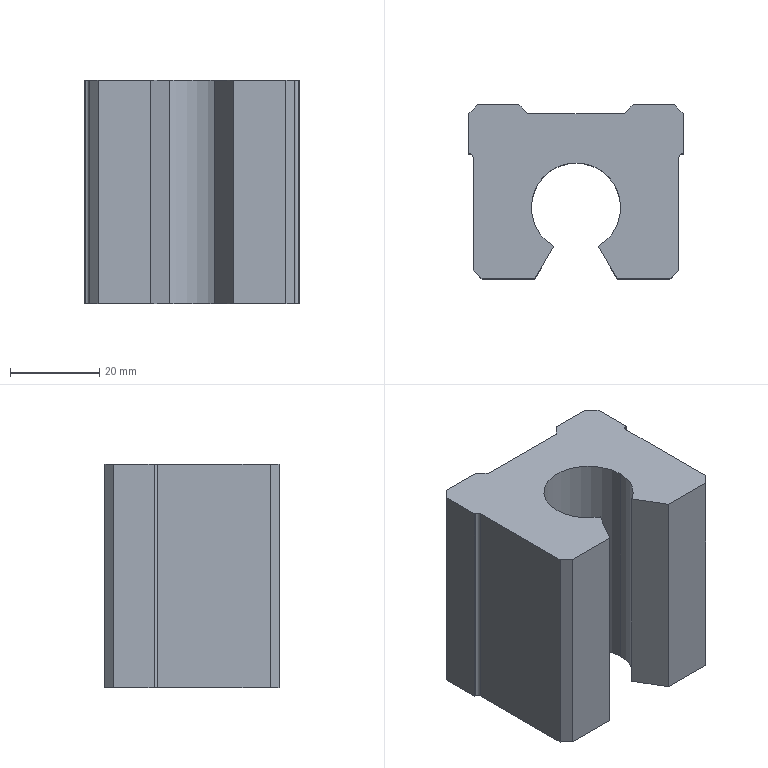Part | SolidWorks | features Chamfer 1, Extrusion 1, ICE 1 | 1 solid | 42 faces | box 48 x 39 x 50 mm | volume 66905 mm3 | plane 21 | cylinder 13 | cone 8 | commonest cylinder face diameters 4.891 x8 20 x3 1.536 x2
STEP:
#1=CARTESIAN_POINT('',(17.5,38.,-42.5));
#2=VERTEX_POINT('',#1);
#3=CARTESIAN_POINT('',(17.5,40.445,-40.054));
#4=VERTEX_POINT('',#3);
#5=CARTESIAN_POINT('',(17.5,40.445,-40.054));
#6=DIRECTION('',(0.,0.7071,0.7071));
#7=VECTOR('',#6,1000.);
#8=LINE('',#5,#7);
#9=EDGE_CURVE('',#2,#4,#8,.T.);
#10=ORIENTED_EDGE('',*,*,#9,.F.);
#11=CARTESIAN_POINT('',(17.5,40.445,-44.945));
#12=VERTEX_POINT('',#11);
#13=CARTESIAN_POINT('',(17.5,40.445,-44.945));
#14=DIRECTION('',(0.,0.7071,-0.7071));
#15=VECTOR('',#14,1000.);
#16=LINE('',#13,#15);
#17=EDGE_CURVE('',#2,#12,#16,.T.);
#18=ORIENTED_EDGE('',*,*,#17,.T.);
#19=CARTESIAN_POINT('',(17.5,40.445,-42.5));
#20=DIRECTION('',(0.,-1.,0.));
#21=DIRECTION('',(0.,0.,1.));
#22=AXIS2_PLACEMENT_3D('',#19,#20,#21);
#23=CIRCLE('',#22,2.445);
#24=EDGE_CURVE('',#4,#12,#23,.T.);
#25=ORIENTED_EDGE('',*,*,#24,.F.);
#26=EDGE_LOOP('',(#10,#18,#25));
#27=FACE_OUTER_BOUND('',#26,.T.);
#28=CARTESIAN_POINT('',(17.5,40.445,-42.5));
#29=DIRECTION('',(0.,1.,0.));
#30=DIRECTION('',(0.,0.,1.));
#31=AXIS2_PLACEMENT_3D('',#28,#29,#30);
#32=CONICAL_SURFACE('',#31,2.446,0.7854);
#33=ADVANCED_FACE('',(#27),#32,.F.);
#34=CARTESIAN_POINT('',(-17.5,38.,-42.5));
#35=VERTEX_POINT('',#34);
#36=CARTESIAN_POINT('',(-17.5,40.445,-40.055));
#37=VERTEX_POINT('',#36);
#38=CARTESIAN_POINT('',(-17.5,40.445,-40.055));
#39=DIRECTION('',(0.,0.7071,0.7071));
#40=VECTOR('',#39,1000.);
#41=LINE('',#38,#40);
#42=EDGE_CURVE('',#35,#37,#41,.T.);
#43=ORIENTED_EDGE('',*,*,#42,.F.);
#44=CARTESIAN_POINT('',(-17.5,40.445,-44.946));
#45=VERTEX_POINT('',#44);
#46=CARTESIAN_POINT('',(-17.5,40.445,-44.946));
#47=DIRECTION('',(0.,0.7071,-0.7071));
#48=VECTOR('',#47,1000.);
#49=LINE('',#46,#48);
#50=EDGE_CURVE('',#35,#45,#49,.T.);
#51=ORIENTED_EDGE('',*,*,#50,.T.);
#52=CARTESIAN_POINT('',(-17.5,40.445,-42.5));
#53=DIRECTION('',(0.,-1.,0.));
#54=DIRECTION('',(0.,0.,1.));
#55=AXIS2_PLACEMENT_3D('',#52,#53,#54);
#56=CIRCLE('',#55,2.446);
#57=EDGE_CURVE('',#37,#45,#56,.T.);
#58=ORIENTED_EDGE('',*,*,#57,.F.);
#59=EDGE_LOOP('',(#43,#51,#58));
#60=FACE_OUTER_BOUND('',#59,.T.);
#61=CARTESIAN_POINT('',(-17.5,40.445,-42.5));
#62=DIRECTION('',(0.,1.,0.));
#63=DIRECTION('',(0.,0.,1.));
#64=AXIS2_PLACEMENT_3D('',#61,#62,#63);
#65=CONICAL_SURFACE('',#64,2.446,0.7854);
#66=ADVANCED_FACE('',(#60),#65,.F.);
#67=CARTESIAN_POINT('',(-17.5,38.,-7.5));
#68=VERTEX_POINT('',#67);
#69=CARTESIAN_POINT('',(-17.5,40.446,-5.054));
#70=VERTEX_POINT('',#69);
#71=CARTESIAN_POINT('',(-17.5,40.446,-5.054));
#72=DIRECTION('',(0.,0.7071,0.7071));
#73=VECTOR('',#72,1000.);
#74=LINE('',#71,#73);
#75=EDGE_CURVE('',#68,#70,#74,.T.);
#76=ORIENTED_EDGE('',*,*,#75,.F.);
#77=CARTESIAN_POINT('',(-17.5,40.446,-9.945));
#78=VERTEX_POINT('',#77);
#79=CARTESIAN_POINT('',(-17.5,40.446,-9.945));
#80=DIRECTION('',(0.,0.7071,-0.7071));
#81=VECTOR('',#80,1000.);
#82=LINE('',#79,#81);
#83=EDGE_CURVE('',#68,#78,#82,.T.);
#84=ORIENTED_EDGE('',*,*,#83,.T.);
#85=CARTESIAN_POINT('',(-17.5,40.446,-7.5));
#86=DIRECTION('',(0.,-1.,0.));
#87=DIRECTION('',(0.,0.,1.));
#88=AXIS2_PLACEMENT_3D('',#85,#86,#87);
#89=CIRCLE('',#88,2.445);
#90=EDGE_CURVE('',#70,#78,#89,.T.);
#91=ORIENTED_EDGE('',*,*,#90,.F.);
#92=EDGE_LOOP('',(#76,#84,#91));
#93=FACE_OUTER_BOUND('',#92,.T.);
#94=CARTESIAN_POINT('',(-17.5,40.446,-7.5));
#95=DIRECTION('',(0.,1.,0.));
#96=DIRECTION('',(0.,0.,1.));
#97=AXIS2_PLACEMENT_3D('',#94,#95,#96);
#98=CONICAL_SURFACE('',#97,2.446,0.7854);
#99=ADVANCED_FACE('',(#93),#98,.F.);
#100=CARTESIAN_POINT('',(17.5,38.,-7.5));
#101=VERTEX_POINT('',#100);
#102=CARTESIAN_POINT('',(17.5,40.445,-5.055));
#103=VERTEX_POINT('',#102);
#104=CARTESIAN_POINT('',(17.5,40.445,-5.054));
#105=DIRECTION('',(0.,0.7071,0.7071));
#106=VECTOR('',#105,1000.);
#107=LINE('',#104,#106);
#108=EDGE_CURVE('',#101,#103,#107,.T.);
#109=ORIENTED_EDGE('',*,*,#108,.F.);
#110=CARTESIAN_POINT('',(17.5,40.445,-9.946));
#111=VERTEX_POINT('',#110);
#112=CARTESIAN_POINT('',(17.5,40.445,-9.946));
#113=DIRECTION('',(0.,0.7071,-0.7071));
#114=VECTOR('',#113,1000.);
#115=LINE('',#112,#114);
#116=EDGE_CURVE('',#101,#111,#115,.T.);
#117=ORIENTED_EDGE('',*,*,#116,.T.);
#118=CARTESIAN_POINT('',(17.5,40.445,-7.5));
#119=DIRECTION('',(0.,-1.,0.));
#120=DIRECTION('',(0.,0.,1.));
#121=AXIS2_PLACEMENT_3D('',#118,#119,#120);
#122=CIRCLE('',#121,2.445);
#123=EDGE_CURVE('',#103,#111,#122,.T.);
#124=ORIENTED_EDGE('',*,*,#123,.F.);
#125=EDGE_LOOP('',(#109,#117,#124));
#126=FACE_OUTER_BOUND('',#125,.T.);
#127=CARTESIAN_POINT('',(17.5,40.445,-7.5));
#128=DIRECTION('',(0.,1.,0.));
#129=DIRECTION('',(0.,0.,1.));
#130=AXIS2_PLACEMENT_3D('',#127,#128,#129);
#131=CONICAL_SURFACE('',#130,2.446,0.7854);
#132=ADVANCED_FACE('',(#126),#131,.F.);
#133=ORIENTED_EDGE('',*,*,#123,.T.);
#134=CARTESIAN_POINT('',(17.5,50.,-9.946));
#135=VERTEX_POINT('',#134);
#136=CARTESIAN_POINT('',(17.5,38.,-9.945));
#137=DIRECTION('',(0.,1.,0.));
#138=VECTOR('',#137,1000.);
#139=LINE('',#136,#138);
#140=EDGE_CURVE('',#111,#135,#139,.T.);
#141=ORIENTED_EDGE('',*,*,#140,.T.);
#142=CARTESIAN_POINT('',(17.5,50.,-5.055));
#143=VERTEX_POINT('',#142);
#144=CARTESIAN_POINT('',(17.5,50.,-7.5));
#145=DIRECTION('',(0.,1.,0.));
#146=DIRECTION('',(0.,0.,1.));
#147=AXIS2_PLACEMENT_3D('',#144,#145,#146);
#148=CIRCLE('',#147,2.445);
#149=EDGE_CURVE('',#135,#143,#148,.T.);
#150=ORIENTED_EDGE('',*,*,#149,.T.);
#151=CARTESIAN_POINT('',(17.5,38.,-5.054));
#152=DIRECTION('',(0.,1.,0.));
#153=VECTOR('',#152,1000.);
#154=LINE('',#151,#153);
#155=EDGE_CURVE('',#103,#143,#154,.T.);
#156=ORIENTED_EDGE('',*,*,#155,.F.);
#157=EDGE_LOOP('',(#133,#141,#150,#156));
#158=FACE_OUTER_BOUND('',#157,.T.);
#159=CARTESIAN_POINT('',(17.5,38.,-7.5));
#160=DIRECTION('',(0.,1.,0.));
#161=DIRECTION('',(0.,0.,1.));
#162=AXIS2_PLACEMENT_3D('',#159,#160,#161);
#163=CYLINDRICAL_SURFACE('',#162,2.445);
#164=ADVANCED_FACE('',(#158),#163,.F.);
#165=ORIENTED_EDGE('',*,*,#24,.T.);
#166=CARTESIAN_POINT('',(17.5,50.,-44.945));
#167=VERTEX_POINT('',#166);
#168=CARTESIAN_POINT('',(17.5,38.,-44.945));
#169=DIRECTION('',(0.,1.,0.));
#170=VECTOR('',#169,1000.);
#171=LINE('',#168,#170);
#172=EDGE_CURVE('',#12,#167,#171,.T.);
#173=ORIENTED_EDGE('',*,*,#172,.T.);
#174=CARTESIAN_POINT('',(17.5,50.,-40.054));
#175=VERTEX_POINT('',#174);
#176=CARTESIAN_POINT('',(17.5,50.,-42.5));
#177=DIRECTION('',(0.,1.,0.));
#178=DIRECTION('',(0.,0.,1.));
#179=AXIS2_PLACEMENT_3D('',#176,#177,#178);
#180=CIRCLE('',#179,2.445);
#181=EDGE_CURVE('',#167,#175,#180,.T.);
#182=ORIENTED_EDGE('',*,*,#181,.T.);
#183=CARTESIAN_POINT('',(17.5,38.,-40.054));
#184=DIRECTION('',(0.,1.,0.));
#185=VECTOR('',#184,1000.);
#186=LINE('',#183,#185);
#187=EDGE_CURVE('',#4,#175,#186,.T.);
#188=ORIENTED_EDGE('',*,*,#187,.F.);
#189=EDGE_LOOP('',(#165,#173,#182,#188));
#190=FACE_OUTER_BOUND('',#189,.T.);
#191=CARTESIAN_POINT('',(17.5,38.,-42.5));
#192=DIRECTION('',(0.,1.,0.));
#193=DIRECTION('',(0.,0.,1.));
#194=AXIS2_PLACEMENT_3D('',#191,#192,#193);
#195=CYLINDRICAL_SURFACE('',#194,2.445);
#196=ADVANCED_FACE('',(#190),#195,.F.);
#197=ORIENTED_EDGE('',*,*,#57,.T.);
#198=CARTESIAN_POINT('',(-17.5,50.,-44.945));
#199=VERTEX_POINT('',#198);
#200=CARTESIAN_POINT('',(-17.5,38.,-44.945));
#201=DIRECTION('',(0.,1.,0.));
#202=VECTOR('',#201,1000.);
#203=LINE('',#200,#202);
#204=EDGE_CURVE('',#45,#199,#203,.T.);
#205=ORIENTED_EDGE('',*,*,#204,.T.);
#206=CARTESIAN_POINT('',(-17.5,50.,-40.054));
#207=VERTEX_POINT('',#206);
#208=CARTESIAN_POINT('',(-17.5,50.,-42.5));
#209=DIRECTION('',(0.,1.,0.));
#210=DIRECTION('',(0.,0.,1.));
#211=AXIS2_PLACEMENT_3D('',#208,#209,#210);
#212=CIRCLE('',#211,2.446);
#213=EDGE_CURVE('',#199,#207,#212,.T.);
#214=ORIENTED_EDGE('',*,*,#213,.T.);
#215=CARTESIAN_POINT('',(-17.5,38.,-40.054));
#216=DIRECTION('',(0.,1.,0.));
#217=VECTOR('',#216,1000.);
#218=LINE('',#215,#217);
#219=EDGE_CURVE('',#37,#207,#218,.T.);
#220=ORIENTED_EDGE('',*,*,#219,.F.);
#221=EDGE_LOOP('',(#197,#205,#214,#220));
#222=FACE_OUTER_BOUND('',#221,.T.);
#223=CARTESIAN_POINT('',(-17.5,38.,-42.5));
#224=DIRECTION('',(0.,1.,0.));
#225=DIRECTION('',(0.,0.,1.));
#226=AXIS2_PLACEMENT_3D('',#223,#224,#225);
#227=CYLINDRICAL_SURFACE('',#226,2.446);
#228=ADVANCED_FACE('',(#222),#227,.F.);
#229=ORIENTED_EDGE('',*,*,#90,.T.);
#230=CARTESIAN_POINT('',(-17.5,50.,-9.945));
#231=VERTEX_POINT('',#230);
#232=CARTESIAN_POINT('',(-17.5,38.,-9.945));
#233=DIRECTION('',(0.,1.,0.));
#234=VECTOR('',#233,1000.);
#235=LINE('',#232,#234);
#236=EDGE_CURVE('',#78,#231,#235,.T.);
#237=ORIENTED_EDGE('',*,*,#236,.T.);
#238=CARTESIAN_POINT('',(-17.5,50.,-5.054));
#239=VERTEX_POINT('',#238);
#240=CARTESIAN_POINT('',(-17.5,50.,-7.5));
#241=DIRECTION('',(0.,1.,0.));
#242=DIRECTION('',(0.,0.,1.));
#243=AXIS2_PLACEMENT_3D('',#240,#241,#242);
#244=CIRCLE('',#243,2.445);
#245=EDGE_CURVE('',#231,#239,#244,.T.);
#246=ORIENTED_EDGE('',*,*,#245,.T.);
#247=CARTESIAN_POINT('',(-17.5,38.,-5.054));
#248=DIRECTION('',(0.,1.,0.));
#249=VECTOR('',#248,1000.);
#250=LINE('',#247,#249);
#251=EDGE_CURVE('',#70,#239,#250,.T.);
#252=ORIENTED_EDGE('',*,*,#251,.F.);
#253=EDGE_LOOP('',(#229,#237,#246,#252));
#254=FACE_OUTER_BOUND('',#253,.T.);
#255=CARTESIAN_POINT('',(-17.5,38.,-7.5));
#256=DIRECTION('',(0.,1.,0.));
#257=DIRECTION('',(0.,0.,1.));
#258=AXIS2_PLACEMENT_3D('',#255,#256,#257);
#259=CYLINDRICAL_SURFACE('',#258,2.445);
#260=ADVANCED_FACE('',(#254),#259,.F.);
#261=CARTESIAN_POINT('',(-5.,18.34,-50.));
#262=VERTEX_POINT('',#261);
#263=CARTESIAN_POINT('',(-10.,27.,-50.));
#264=VERTEX_POINT('',#263);
#265=CARTESIAN_POINT('',(0.,27.,-50.));
#266=DIRECTION('',(0.,0.,-1.));
#267=DIRECTION('',(1.,0.,0.));
#268=AXIS2_PLACEMENT_3D('',#265,#266,#267);
#269=CIRCLE('',#268,10.);
#270=EDGE_CURVE('',#262,#264,#269,.T.);
#271=ORIENTED_EDGE('',*,*,#270,.T.);
#272=CARTESIAN_POINT('',(-10.,27.,0.));
#273=VERTEX_POINT('',#272);
#274=CARTESIAN_POINT('',(-10.,27.,-50.));
#275=DIRECTION('',(0.,0.,1.));
#276=VECTOR('',#275,1000.);
#277=LINE('',#274,#276);
#278=EDGE_CURVE('',#264,#273,#277,.T.);
#279=ORIENTED_EDGE('',*,*,#278,.T.);
#280=CARTESIAN_POINT('',(-5.,18.34,0.));
#281=VERTEX_POINT('',#280);
#282=CARTESIAN_POINT('',(0.,27.,0.));
#283=DIRECTION('',(0.,0.,-1.));
#284=DIRECTION('',(1.,0.,0.));
#285=AXIS2_PLACEMENT_3D('',#282,#283,#284);
#286=CIRCLE('',#285,10.);
#287=EDGE_CURVE('',#281,#273,#286,.T.);
#288=ORIENTED_EDGE('',*,*,#287,.F.);
#289=CARTESIAN_POINT('',(-5.,18.34,-50.));
#290=DIRECTION('',(0.,0.,1.));
#291=VECTOR('',#290,1000.);
#292=LINE('',#289,#291);
#293=EDGE_CURVE('',#262,#281,#292,.T.);
#294=ORIENTED_EDGE('',*,*,#293,.F.);
#295=EDGE_LOOP('',(#271,#279,#288,#294));
#296=FACE_OUTER_BOUND('',#295,.T.);
#297=CARTESIAN_POINT('',(0.,27.,-50.));
#298=DIRECTION('',(0.,0.,1.));
#299=DIRECTION('',(1.,0.,0.));
#300=AXIS2_PLACEMENT_3D('',#297,#298,#299);
#301=CYLINDRICAL_SURFACE('',#300,10.);
#302=ADVANCED_FACE('',(#296),#301,.F.);
#303=ORIENTED_EDGE('',*,*,#278,.F.);
#304=CARTESIAN_POINT('',(10.,27.,-50.));
#305=VERTEX_POINT('',#304);
#306=CARTESIAN_POINT('',(0.,27.,-50.));
#307=DIRECTION('',(0.,0.,-1.));
#308=DIRECTION('',(1.,0.,0.));
#309=AXIS2_PLACEMENT_3D('',#306,#307,#308);
#310=CIRCLE('',#309,10.);
#311=EDGE_CURVE('',#264,#305,#310,.T.);
#312=ORIENTED_EDGE('',*,*,#311,.T.);
#313=CARTESIAN_POINT('',(10.,27.,0.));
#314=VERTEX_POINT('',#313);
#315=CARTESIAN_POINT('',(10.,27.,-50.));
#316=DIRECTION('',(0.,0.,1.));
#317=VECTOR('',#316,1000.);
#318=LINE('',#315,#317);
#319=EDGE_CURVE('',#305,#314,#318,.T.);
#320=ORIENTED_EDGE('',*,*,#319,.T.);
#321=CARTESIAN_POINT('',(0.,27.,0.));
#322=DIRECTION('',(0.,0.,-1.));
#323=DIRECTION('',(1.,0.,0.));
#324=AXIS2_PLACEMENT_3D('',#321,#322,#323);
#325=CIRCLE('',#324,10.);
#326=EDGE_CURVE('',#273,#314,#325,.T.);
#327=ORIENTED_EDGE('',*,*,#326,.F.);
#328=EDGE_LOOP('',(#303,#312,#320,#327));
#329=FACE_OUTER_BOUND('',#328,.T.);
#330=CARTESIAN_POINT('',(0.,27.,-50.));
#331=DIRECTION('',(0.,0.,1.));
#332=DIRECTION('',(1.,0.,0.));
#333=AXIS2_PLACEMENT_3D('',#330,#331,#332);
#334=CYLINDRICAL_SURFACE('',#333,10.);
#335=ADVANCED_FACE('',(#329),#334,.F.);
#336=ORIENTED_EDGE('',*,*,#319,.F.);
#337=CARTESIAN_POINT('',(5.,18.34,-50.));
#338=VERTEX_POINT('',#337);
#339=CARTESIAN_POINT('',(0.,27.,-50.));
#340=DIRECTION('',(0.,0.,-1.));
#341=DIRECTION('',(1.,0.,0.));
#342=AXIS2_PLACEMENT_3D('',#339,#340,#341);
#343=CIRCLE('',#342,10.);
#344=EDGE_CURVE('',#305,#338,#343,.T.);
#345=ORIENTED_EDGE('',*,*,#344,.T.);
#346=CARTESIAN_POINT('',(5.,18.34,0.));
#347=VERTEX_POINT('',#346);
#348=CARTESIAN_POINT('',(5.,18.34,-50.));
#349=DIRECTION('',(0.,0.,1.));
#350=VECTOR('',#349,1000.);
#351=LINE('',#348,#350);
#352=EDGE_CURVE('',#338,#347,#351,.T.);
#353=ORIENTED_EDGE('',*,*,#352,.T.);
#354=CARTESIAN_POINT('',(0.,27.,0.));
#355=DIRECTION('',(0.,0.,-1.));
#356=DIRECTION('',(1.,0.,0.));
#357=AXIS2_PLACEMENT_3D('',#354,#355,#356);
#358=CIRCLE('',#357,10.);
#359=EDGE_CURVE('',#314,#347,#358,.T.);
#360=ORIENTED_EDGE('',*,*,#359,.F.);
#361=EDGE_LOOP('',(#336,#345,#353,#360));
#362=FACE_OUTER_BOUND('',#361,.T.);
#363=CARTESIAN_POINT('',(0.,27.,-50.));
#364=DIRECTION('',(0.,0.,1.));
#365=DIRECTION('',(1.,0.,0.));
#366=AXIS2_PLACEMENT_3D('',#363,#364,#365);
#367=CYLINDRICAL_SURFACE('',#366,10.);
#368=ADVANCED_FACE('',(#362),#367,.F.);
#369=CARTESIAN_POINT('',(-9.238,11.,0.));
#370=VERTEX_POINT('',#369);
#371=CARTESIAN_POINT('',(-5.,18.34,0.));
#372=DIRECTION('',(0.5,0.866,0.));
#373=VECTOR('',#372,1000.);
#374=LINE('',#371,#373);
#375=EDGE_CURVE('',#370,#281,#374,.T.);
#376=ORIENTED_EDGE('',*,*,#375,.F.);
#377=CARTESIAN_POINT('',(-9.238,11.,-50.));
#378=VERTEX_POINT('',#377);
#379=CARTESIAN_POINT('',(-9.238,11.,-50.));
#380=DIRECTION('',(0.,0.,1.));
#381=VECTOR('',#380,1000.);
#382=LINE('',#379,#381);
#383=EDGE_CURVE('',#378,#370,#382,.T.);
#384=ORIENTED_EDGE('',*,*,#383,.F.);
#385=CARTESIAN_POINT('',(-5.,18.34,-50.));
#386=DIRECTION('',(0.5,0.866,0.));
#387=VECTOR('',#386,1000.);
#388=LINE('',#385,#387);
#389=EDGE_CURVE('',#378,#262,#388,.T.);
#390=ORIENTED_EDGE('',*,*,#389,.T.);
#391=ORIENTED_EDGE('',*,*,#293,.T.);
#392=EDGE_LOOP('',(#376,#384,#390,#391));
#393=FACE_OUTER_BOUND('',#392,.T.);
#394=CARTESIAN_POINT('',(-5.,18.34,-50.));
#395=DIRECTION('',(0.866,-0.5,0.));
#396=DIRECTION('',(0.5,0.866,0.));
#397=AXIS2_PLACEMENT_3D('',#394,#395,#396);
#398=PLANE('',#397);
#399=ADVANCED_FACE('',(#393),#398,.T.);
#400=CARTESIAN_POINT('',(-21.04,11.,0.));
#401=VERTEX_POINT('',#400);
#402=CARTESIAN_POINT('',(-9.238,11.,0.));
#403=DIRECTION('',(1.,0.,0.));
#404=VECTOR('',#403,1000.);
#405=LINE('',#402,#404);
#406=EDGE_CURVE('',#401,#370,#405,.T.);
#407=ORIENTED_EDGE('',*,*,#406,.F.);
#408=CARTESIAN_POINT('',(-21.04,11.,-50.));
#409=VERTEX_POINT('',#408);
#410=CARTESIAN_POINT('',(-21.04,11.,-50.));
#411=DIRECTION('',(0.,0.,1.));
#412=VECTOR('',#411,1000.);
#413=LINE('',#410,#412);
#414=EDGE_CURVE('',#409,#401,#413,.T.);
#415=ORIENTED_EDGE('',*,*,#414,.F.);
#416=CARTESIAN_POINT('',(-9.238,11.,-50.));
#417=DIRECTION('',(1.,0.,0.));
#418=VECTOR('',#417,1000.);
#419=LINE('',#416,#418);
#420=EDGE_CURVE('',#409,#378,#419,.T.);
#421=ORIENTED_EDGE('',*,*,#420,.T.);
#422=ORIENTED_EDGE('',*,*,#383,.T.);
#423=EDGE_LOOP('',(#407,#415,#421,#422));
#424=FACE_OUTER_BOUND('',#423,.T.);
#425=CARTESIAN_POINT('',(-9.238,11.,-50.));
#426=DIRECTION('',(0.,-1.,0.));
#427=DIRECTION('',(0.,0.,-1.));
#428=AXIS2_PLACEMENT_3D('',#425,#426,#427);
#429=PLANE('',#428);
#430=ADVANCED_FACE('',(#424),#429,.T.);
#431=CARTESIAN_POINT('',(-23.04,13.,0.));
#432=VERTEX_POINT('',#431);
#433=CARTESIAN_POINT('',(-23.04,13.,0.));
#434=DIRECTION('',(0.7071,-0.7071,0.));
#435=VECTOR('',#434,1000.);
#436=LINE('',#433,#435);
#437=EDGE_CURVE('',#432,#401,#436,.T.);
#438=ORIENTED_EDGE('',*,*,#437,.F.);
#439=CARTESIAN_POINT('',(-23.04,13.,-50.));
#440=VERTEX_POINT('',#439);
#441=CARTESIAN_POINT('',(-23.04,13.,-50.));
#442=DIRECTION('',(0.,0.,1.));
#443=VECTOR('',#442,1000.);
#444=LINE('',#441,#443);
#445=EDGE_CURVE('',#440,#432,#444,.T.);
#446=ORIENTED_EDGE('',*,*,#445,.F.);
#447=CARTESIAN_POINT('',(-23.04,13.,-50.));
#448=DIRECTION('',(0.7071,-0.7071,0.));
#449=VECTOR('',#448,1000.);
#450=LINE('',#447,#449);
#451=EDGE_CURVE('',#440,#409,#450,.T.);
#452=ORIENTED_EDGE('',*,*,#451,.T.);
#453=ORIENTED_EDGE('',*,*,#414,.T.);
#454=EDGE_LOOP('',(#438,#446,#452,#453));
#455=FACE_OUTER_BOUND('',#454,.T.);
#456=CARTESIAN_POINT('',(-23.04,13.,-50.));
#457=DIRECTION('',(-0.7071,-0.7071,0.));
#458=DIRECTION('',(0.7071,-0.7071,0.));
#459=AXIS2_PLACEMENT_3D('',#456,#457,#458);
#460=PLANE('',#459);
#461=ADVANCED_FACE('',(#455),#460,.T.);
#462=CARTESIAN_POINT('',(-23.04,38.232,0.));
#463=VERTEX_POINT('',#462);
#464=CARTESIAN_POINT('',(-23.04,13.,0.));
#465=DIRECTION('',(0.,-1.,0.));
#466=VECTOR('',#465,1000.);
#467=LINE('',#464,#466);
#468=EDGE_CURVE('',#463,#432,#467,.T.);
#469=ORIENTED_EDGE('',*,*,#468,.F.);
#470=CARTESIAN_POINT('',(-23.04,38.232,-50.));
#471=VERTEX_POINT('',#470);
#472=CARTESIAN_POINT('',(-23.04,38.232,-50.));
#473=DIRECTION('',(0.,0.,1.));
#474=VECTOR('',#473,1000.);
#475=LINE('',#472,#474);
#476=EDGE_CURVE('',#471,#463,#475,.T.);
#477=ORIENTED_EDGE('',*,*,#476,.F.);
#478=CARTESIAN_POINT('',(-23.04,13.,-50.));
#479=DIRECTION('',(0.,-1.,0.));
#480=VECTOR('',#479,1000.);
#481=LINE('',#478,#480);
#482=EDGE_CURVE('',#471,#440,#481,.T.);
#483=ORIENTED_EDGE('',*,*,#482,.T.);
#484=ORIENTED_EDGE('',*,*,#445,.T.);
#485=EDGE_LOOP('',(#469,#477,#483,#484));
#486=FACE_OUTER_BOUND('',#485,.T.);
#487=CARTESIAN_POINT('',(-23.04,13.,-50.));
#488=DIRECTION('',(-1.,0.,0.));
#489=DIRECTION('',(0.,0.,1.));
#490=AXIS2_PLACEMENT_3D('',#487,#488,#489);
#491=PLANE('',#490);
#492=ADVANCED_FACE('',(#486),#491,.T.);
#493=CARTESIAN_POINT('',(-23.808,39.,0.));
#494=VERTEX_POINT('',#493);
#495=CARTESIAN_POINT('',(-23.808,38.232,0.));
#496=DIRECTION('',(0.,0.,-1.));
#497=DIRECTION('',(1.,0.,0.));
#498=AXIS2_PLACEMENT_3D('',#495,#496,#497);
#499=CIRCLE('',#498,0.768);
#500=EDGE_CURVE('',#494,#463,#499,.T.);
#501=ORIENTED_EDGE('',*,*,#500,.F.);
#502=CARTESIAN_POINT('',(-23.808,39.,-50.));
#503=VERTEX_POINT('',#502);
#504=CARTESIAN_POINT('',(-23.808,39.,-50.));
#505=DIRECTION('',(0.,0.,1.));
#506=VECTOR('',#505,1000.);
#507=LINE('',#504,#506);
#508=EDGE_CURVE('',#503,#494,#507,.T.);
#509=ORIENTED_EDGE('',*,*,#508,.F.);
#510=CARTESIAN_POINT('',(-23.808,38.232,-50.));
#511=DIRECTION('',(0.,0.,-1.));
#512=DIRECTION('',(1.,0.,0.));
#513=AXIS2_PLACEMENT_3D('',#510,#511,#512);
#514=CIRCLE('',#513,0.768);
#515=EDGE_CURVE('',#503,#471,#514,.T.);
#516=ORIENTED_EDGE('',*,*,#515,.T.);
#517=ORIENTED_EDGE('',*,*,#476,.T.);
#518=EDGE_LOOP('',(#501,#509,#516,#517));
#519=FACE_OUTER_BOUND('',#518,.T.);
#520=CARTESIAN_POINT('',(-23.808,38.232,-50.));
#521=DIRECTION('',(0.,0.,1.));
#522=DIRECTION('',(1.,0.,0.));
#523=AXIS2_PLACEMENT_3D('',#520,#521,#522);
#524=CYLINDRICAL_SURFACE('',#523,0.768);
#525=ADVANCED_FACE('',(#519),#524,.F.);
#526=CARTESIAN_POINT('',(-24.,39.,0.));
#527=VERTEX_POINT('',#526);
#528=CARTESIAN_POINT('',(-23.808,39.,0.));
#529=DIRECTION('',(1.,0.,0.));
#530=VECTOR('',#529,1000.);
#531=LINE('',#528,#530);
#532=EDGE_CURVE('',#527,#494,#531,.T.);
#533=ORIENTED_EDGE('',*,*,#532,.F.);
#534=CARTESIAN_POINT('',(-24.,39.,-50.));
#535=VERTEX_POINT('',#534);
#536=CARTESIAN_POINT('',(-24.,39.,-50.));
#537=DIRECTION('',(0.,0.,1.));
#538=VECTOR('',#537,1000.);
#539=LINE('',#536,#538);
#540=EDGE_CURVE('',#535,#527,#539,.T.);
#541=ORIENTED_EDGE('',*,*,#540,.F.);
#542=CARTESIAN_POINT('',(-23.808,39.,-50.));
#543=DIRECTION('',(1.,0.,0.));
#544=VECTOR('',#543,1000.);
#545=LINE('',#542,#544);
#546=EDGE_CURVE('',#535,#503,#545,.T.);
#547=ORIENTED_EDGE('',*,*,#546,.T.);
#548=ORIENTED_EDGE('',*,*,#508,.T.);
#549=EDGE_LOOP('',(#533,#541,#547,#548));
#550=FACE_OUTER_BOUND('',#549,.T.);
#551=CARTESIAN_POINT('',(-23.808,39.,-50.));
#552=DIRECTION('',(0.,-1.,0.));
#553=DIRECTION('',(0.,0.,-1.));
#554=AXIS2_PLACEMENT_3D('',#551,#552,#553);
#555=PLANE('',#554);
#556=ADVANCED_FACE('',(#550),#555,.T.);
#557=CARTESIAN_POINT('',(-24.,48.,0.));
#558=VERTEX_POINT('',#557);
#559=CARTESIAN_POINT('',(-24.,39.,0.));
#560=DIRECTION('',(0.,-1.,0.));
#561=VECTOR('',#560,1000.);
#562=LINE('',#559,#561);
#563=EDGE_CURVE('',#558,#527,#562,.T.);
#564=ORIENTED_EDGE('',*,*,#563,.F.);
#565=CARTESIAN_POINT('',(-24.,48.,-50.));
#566=VERTEX_POINT('',#565);
#567=CARTESIAN_POINT('',(-24.,48.,-50.));
#568=DIRECTION('',(0.,0.,1.));
#569=VECTOR('',#568,1000.);
#570=LINE('',#567,#569);
#571=EDGE_CURVE('',#566,#558,#570,.T.);
#572=ORIENTED_EDGE('',*,*,#571,.F.);
#573=CARTESIAN_POINT('',(-24.,39.,-50.));
#574=DIRECTION('',(0.,-1.,0.));
#575=VECTOR('',#574,1000.);
#576=LINE('',#573,#575);
#577=EDGE_CURVE('',#566,#535,#576,.T.);
#578=ORIENTED_EDGE('',*,*,#577,.T.);
#579=ORIENTED_EDGE('',*,*,#540,.T.);
#580=EDGE_LOOP('',(#564,#572,#578,#579));
#581=FACE_OUTER_BOUND('',#580,.T.);
#582=CARTESIAN_POINT('',(-24.,39.,-50.));
#583=DIRECTION('',(-1.,0.,0.));
#584=DIRECTION('',(0.,0.,1.));
#585=AXIS2_PLACEMENT_3D('',#582,#583,#584);
#586=PLANE('',#585);
#587=ADVANCED_FACE('',(#581),#586,.T.);
#588=CARTESIAN_POINT('',(-22.,50.,0.));
#589=VERTEX_POINT('',#588);
#590=CARTESIAN_POINT('',(-24.,48.,0.));
#591=DIRECTION('',(-0.7071,-0.7071,0.));
#592=VECTOR('',#591,1000.);
#593=LINE('',#590,#592);
#594=EDGE_CURVE('',#589,#558,#593,.T.);
#595=ORIENTED_EDGE('',*,*,#594,.F.);
#596=CARTESIAN_POINT('',(-22.,50.,-50.));
#597=VERTEX_POINT('',#596);
#598=CARTESIAN_POINT('',(-22.,50.,-50.));
#599=DIRECTION('',(0.,0.,1.));
#600=VECTOR('',#599,1000.);
#601=LINE('',#598,#600);
#602=EDGE_CURVE('',#597,#589,#601,.T.);
#603=ORIENTED_EDGE('',*,*,#602,.F.);
#604=CARTESIAN_POINT('',(-24.,48.,-50.));
#605=DIRECTION('',(-0.7071,-0.7071,0.));
#606=VECTOR('',#605,1000.);
#607=LINE('',#604,#606);
#608=EDGE_CURVE('',#597,#566,#607,.T.);
#609=ORIENTED_EDGE('',*,*,#608,.T.);
#610=ORIENTED_EDGE('',*,*,#571,.T.);
#611=EDGE_LOOP('',(#595,#603,#609,#610));
#612=FACE_OUTER_BOUND('',#611,.T.);
#613=CARTESIAN_POINT('',(-24.,48.,-50.));
#614=DIRECTION('',(-0.7071,0.7071,0.));
#615=DIRECTION('',(-0.7071,-0.7071,0.));
#616=AXIS2_PLACEMENT_3D('',#613,#614,#615);
#617=PLANE('',#616);
#618=ADVANCED_FACE('',(#612),#617,.T.);
#619=CARTESIAN_POINT('',(-17.5,50.,-42.5));
#620=DIRECTION('',(0.,1.,0.));
#621=DIRECTION('',(0.,0.,1.));
#622=AXIS2_PLACEMENT_3D('',#619,#620,#621);
#623=CIRCLE('',#622,2.446);
#624=EDGE_CURVE('',#207,#199,#623,.T.);
#625=ORIENTED_EDGE('',*,*,#624,.F.);
#626=ORIENTED_EDGE('',*,*,#213,.F.);
#627=EDGE_LOOP('',(#625,#626));
#628=FACE_BOUND('',#627,.T.);
#629=CARTESIAN_POINT('',(-17.5,50.,-7.5));
#630=DIRECTION('',(0.,1.,0.));
#631=DIRECTION('',(0.,0.,1.));
#632=AXIS2_PLACEMENT_3D('',#629,#630,#631);
#633=CIRCLE('',#632,2.445);
#634=EDGE_CURVE('',#239,#231,#633,.T.);
#635=ORIENTED_EDGE('',*,*,#634,.F.);
#636=ORIENTED_EDGE('',*,*,#245,.F.);
#637=EDGE_LOOP('',(#635,#636));
#638=FACE_BOUND('',#637,.T.);
#639=CARTESIAN_POINT('',(-12.8,50.,0.));
#640=VERTEX_POINT('',#639);
#641=CARTESIAN_POINT('',(-22.,50.,0.));
#642=DIRECTION('',(-1.,0.,0.));
#643=VECTOR('',#642,1000.);
#644=LINE('',#641,#643);
#645=EDGE_CURVE('',#640,#589,#644,.T.);
#646=ORIENTED_EDGE('',*,*,#645,.F.);
#647=CARTESIAN_POINT('',(-12.8,50.,-50.));
#648=VERTEX_POINT('',#647);
#649=CARTESIAN_POINT('',(-12.8,50.,-50.));
#650=DIRECTION('',(0.,0.,1.));
#651=VECTOR('',#650,1000.);
#652=LINE('',#649,#651);
#653=EDGE_CURVE('',#648,#640,#652,.T.);
#654=ORIENTED_EDGE('',*,*,#653,.F.);
#655=CARTESIAN_POINT('',(-22.,50.,-50.));
#656=DIRECTION('',(-1.,0.,0.));
#657=VECTOR('',#656,1000.);
#658=LINE('',#655,#657);
#659=EDGE_CURVE('',#648,#597,#658,.T.);
#660=ORIENTED_EDGE('',*,*,#659,.T.);
#661=ORIENTED_EDGE('',*,*,#602,.T.);
#662=EDGE_LOOP('',(#646,#654,#660,#661));
#663=FACE_OUTER_BOUND('',#662,.T.);
#664=CARTESIAN_POINT('',(-22.,50.,-50.));
#665=DIRECTION('',(0.,1.,0.));
#666=DIRECTION('',(0.,0.,1.));
#667=AXIS2_PLACEMENT_3D('',#664,#665,#666);
#668=PLANE('',#667);
#669=ADVANCED_FACE('',(#628,#638,#663),#668,.T.);
#670=CARTESIAN_POINT('',(-10.8,48.,0.));
#671=VERTEX_POINT('',#670);
#672=CARTESIAN_POINT('',(-12.8,50.,0.));
#673=DIRECTION('',(-0.7071,0.7071,0.));
#674=VECTOR('',#673,1000.);
#675=LINE('',#672,#674);
#676=EDGE_CURVE('',#671,#640,#675,.T.);
#677=ORIENTED_EDGE('',*,*,#676,.F.);
#678=CARTESIAN_POINT('',(-10.8,48.,-50.));
#679=VERTEX_POINT('',#678);
#680=CARTESIAN_POINT('',(-10.8,48.,-50.));
#681=DIRECTION('',(0.,0.,1.));
#682=VECTOR('',#681,1000.);
#683=LINE('',#680,#682);
#684=EDGE_CURVE('',#679,#671,#683,.T.);
#685=ORIENTED_EDGE('',*,*,#684,.F.);
#686=CARTESIAN_POINT('',(-12.8,50.,-50.));
#687=DIRECTION('',(-0.7071,0.7071,0.));
#688=VECTOR('',#687,1000.);
#689=LINE('',#686,#688);
#690=EDGE_CURVE('',#679,#648,#689,.T.);
#691=ORIENTED_EDGE('',*,*,#690,.T.);
#692=ORIENTED_EDGE('',*,*,#653,.T.);
#693=EDGE_LOOP('',(#677,#685,#691,#692));
#694=FACE_OUTER_BOUND('',#693,.T.);
#695=CARTESIAN_POINT('',(-12.8,50.,-50.));
#696=DIRECTION('',(0.7071,0.7071,0.));
#697=DIRECTION('',(-0.7071,0.7071,0.));
#698=AXIS2_PLACEMENT_3D('',#695,#696,#697);
#699=PLANE('',#698);
#700=ADVANCED_FACE('',(#694),#699,.T.);
#701=CARTESIAN_POINT('',(10.8,48.,0.));
#702=VERTEX_POINT('',#701);
#703=CARTESIAN_POINT('',(-10.8,48.,0.));
#704=DIRECTION('',(-1.,0.,0.));
#705=VECTOR('',#704,1000.);
#706=LINE('',#703,#705);
#707=EDGE_CURVE('',#702,#671,#706,.T.);
#708=ORIENTED_EDGE('',*,*,#707,.F.);
#709=CARTESIAN_POINT('',(10.8,48.,-50.));
#710=VERTEX_POINT('',#709);
#711=CARTESIAN_POINT('',(10.8,48.,-50.));
#712=DIRECTION('',(0.,0.,1.));
#713=VECTOR('',#712,1000.);
#714=LINE('',#711,#713);
#715=EDGE_CURVE('',#710,#702,#714,.T.);
#716=ORIENTED_EDGE('',*,*,#715,.F.);
#717=CARTESIAN_POINT('',(-10.8,48.,-50.));
#718=DIRECTION('',(-1.,0.,0.));
#719=VECTOR('',#718,1000.);
#720=LINE('',#717,#719);
#721=EDGE_CURVE('',#710,#679,#720,.T.);
#722=ORIENTED_EDGE('',*,*,#721,.T.);
#723=ORIENTED_EDGE('',*,*,#684,.T.);
#724=EDGE_LOOP('',(#708,#716,#722,#723));
#725=FACE_OUTER_BOUND('',#724,.T.);
#726=CARTESIAN_POINT('',(-10.8,48.,-50.));
#727=DIRECTION('',(0.,1.,0.));
#728=DIRECTION('',(0.,0.,1.));
#729=AXIS2_PLACEMENT_3D('',#726,#727,#728);
#730=PLANE('',#729);
#731=ADVANCED_FACE('',(#725),#730,.T.);
#732=CARTESIAN_POINT('',(12.8,50.,0.));
#733=VERTEX_POINT('',#732);
#734=CARTESIAN_POINT('',(10.8,48.,0.));
#735=DIRECTION('',(-0.7071,-0.7071,0.));
#736=VECTOR('',#735,1000.);
#737=LINE('',#734,#736);
#738=EDGE_CURVE('',#733,#702,#737,.T.);
#739=ORIENTED_EDGE('',*,*,#738,.F.);
#740=CARTESIAN_POINT('',(12.8,50.,-50.));
#741=VERTEX_POINT('',#740);
#742=CARTESIAN_POINT('',(12.8,50.,-50.));
#743=DIRECTION('',(0.,0.,1.));
#744=VECTOR('',#743,1000.);
#745=LINE('',#742,#744);
#746=EDGE_CURVE('',#741,#733,#745,.T.);
#747=ORIENTED_EDGE('',*,*,#746,.F.);
#748=CARTESIAN_POINT('',(10.8,48.,-50.));
#749=DIRECTION('',(-0.7071,-0.7071,0.));
#750=VECTOR('',#749,1000.);
#751=LINE('',#748,#750);
#752=EDGE_CURVE('',#741,#710,#751,.T.);
#753=ORIENTED_EDGE('',*,*,#752,.T.);
#754=ORIENTED_EDGE('',*,*,#715,.T.);
#755=EDGE_LOOP('',(#739,#747,#753,#754));
#756=FACE_OUTER_BOUND('',#755,.T.);
#757=CARTESIAN_POINT('',(10.8,48.,-50.));
#758=DIRECTION('',(-0.7071,0.7071,0.));
#759=DIRECTION('',(-0.7071,-0.7071,0.));
#760=AXIS2_PLACEMENT_3D('',#757,#758,#759);
#761=PLANE('',#760);
#762=ADVANCED_FACE('',(#756),#761,.T.);
#763=CARTESIAN_POINT('',(17.5,50.,-7.5));
#764=DIRECTION('',(0.,1.,0.));
#765=DIRECTION('',(0.,0.,1.));
#766=AXIS2_PLACEMENT_3D('',#763,#764,#765);
#767=CIRCLE('',#766,2.445);
#768=EDGE_CURVE('',#143,#135,#767,.T.);
#769=ORIENTED_EDGE('',*,*,#768,.F.);
#770=ORIENTED_EDGE('',*,*,#149,.F.);
#771=EDGE_LOOP('',(#769,#770));
#772=FACE_BOUND('',#771,.T.);
#773=CARTESIAN_POINT('',(17.5,50.,-42.5));
#774=DIRECTION('',(0.,1.,0.));
#775=DIRECTION('',(0.,0.,1.));
#776=AXIS2_PLACEMENT_3D('',#773,#774,#775);
#777=CIRCLE('',#776,2.445);
#778=EDGE_CURVE('',#175,#167,#777,.T.);
#779=ORIENTED_EDGE('',*,*,#778,.F.);
#780=ORIENTED_EDGE('',*,*,#181,.F.);
#781=EDGE_LOOP('',(#779,#780));
#782=FACE_BOUND('',#781,.T.);
#783=CARTESIAN_POINT('',(22.,50.,0.));
#784=VERTEX_POINT('',#783);
#785=CARTESIAN_POINT('',(12.8,50.,0.));
#786=DIRECTION('',(-1.,0.,0.));
#787=VECTOR('',#786,1000.);
#788=LINE('',#785,#787);
#789=EDGE_CURVE('',#784,#733,#788,.T.);
#790=ORIENTED_EDGE('',*,*,#789,.F.);
#791=CARTESIAN_POINT('',(22.,50.,-50.));
#792=VERTEX_POINT('',#791);
#793=CARTESIAN_POINT('',(22.,50.,-50.));
#794=DIRECTION('',(0.,0.,1.));
#795=VECTOR('',#794,1000.);
#796=LINE('',#793,#795);
#797=EDGE_CURVE('',#792,#784,#796,.T.);
#798=ORIENTED_EDGE('',*,*,#797,.F.);
#799=CARTESIAN_POINT('',(12.8,50.,-50.));
#800=DIRECTION('',(-1.,0.,0.));
#801=VECTOR('',#800,1000.);
#802=LINE('',#799,#801);
#803=EDGE_CURVE('',#792,#741,#802,.T.);
#804=ORIENTED_EDGE('',*,*,#803,.T.);
#805=ORIENTED_EDGE('',*,*,#746,.T.);
#806=EDGE_LOOP('',(#790,#798,#804,#805));
#807=FACE_OUTER_BOUND('',#806,.T.);
#808=CARTESIAN_POINT('',(12.8,50.,-50.));
#809=DIRECTION('',(0.,1.,0.));
#810=DIRECTION('',(0.,0.,1.));
#811=AXIS2_PLACEMENT_3D('',#808,#809,#810);
#812=PLANE('',#811);
#813=ADVANCED_FACE('',(#772,#782,#807),#812,.T.);
#814=CARTESIAN_POINT('',(24.,48.,0.));
#815=VERTEX_POINT('',#814);
#816=CARTESIAN_POINT('',(22.,50.,0.));
#817=DIRECTION('',(-0.7071,0.7071,0.));
#818=VECTOR('',#817,1000.);
#819=LINE('',#816,#818);
#820=EDGE_CURVE('',#815,#784,#819,.T.);
#821=ORIENTED_EDGE('',*,*,#820,.F.);
#822=CARTESIAN_POINT('',(24.,48.,-50.));
#823=VERTEX_POINT('',#822);
#824=CARTESIAN_POINT('',(24.,48.,-50.));
#825=DIRECTION('',(0.,0.,1.));
#826=VECTOR('',#825,1000.);
#827=LINE('',#824,#826);
#828=EDGE_CURVE('',#823,#815,#827,.T.);
#829=ORIENTED_EDGE('',*,*,#828,.F.);
#830=CARTESIAN_POINT('',(22.,50.,-50.));
#831=DIRECTION('',(-0.7071,0.7071,0.));
#832=VECTOR('',#831,1000.);
#833=LINE('',#830,#832);
#834=EDGE_CURVE('',#823,#792,#833,.T.);
#835=ORIENTED_EDGE('',*,*,#834,.T.);
#836=ORIENTED_EDGE('',*,*,#797,.T.);
#837=EDGE_LOOP('',(#821,#829,#835,#836));
#838=FACE_OUTER_BOUND('',#837,.T.);
#839=CARTESIAN_POINT('',(22.,50.,-50.));
#840=DIRECTION('',(0.7071,0.7071,0.));
#841=DIRECTION('',(-0.7071,0.7071,0.));
#842=AXIS2_PLACEMENT_3D('',#839,#840,#841);
#843=PLANE('',#842);
#844=ADVANCED_FACE('',(#838),#843,.T.);
#845=CARTESIAN_POINT('',(24.,39.,0.));
#846=VERTEX_POINT('',#845);
#847=CARTESIAN_POINT('',(24.,48.,0.));
#848=DIRECTION('',(0.,1.,0.));
#849=VECTOR('',#848,1000.);
#850=LINE('',#847,#849);
#851=EDGE_CURVE('',#846,#815,#850,.T.);
#852=ORIENTED_EDGE('',*,*,#851,.F.);
#853=CARTESIAN_POINT('',(24.,39.,-50.));
#854=VERTEX_POINT('',#853);
#855=CARTESIAN_POINT('',(24.,39.,-50.));
#856=DIRECTION('',(0.,0.,1.));
#857=VECTOR('',#856,1000.);
#858=LINE('',#855,#857);
#859=EDGE_CURVE('',#854,#846,#858,.T.);
#860=ORIENTED_EDGE('',*,*,#859,.F.);
#861=CARTESIAN_POINT('',(24.,48.,-50.));
#862=DIRECTION('',(0.,1.,0.));
#863=VECTOR('',#862,1000.);
#864=LINE('',#861,#863);
#865=EDGE_CURVE('',#854,#823,#864,.T.);
#866=ORIENTED_EDGE('',*,*,#865,.T.);
#867=ORIENTED_EDGE('',*,*,#828,.T.);
#868=EDGE_LOOP('',(#852,#860,#866,#867));
#869=FACE_OUTER_BOUND('',#868,.T.);
#870=CARTESIAN_POINT('',(24.,48.,-50.));
#871=DIRECTION('',(1.,0.,0.));
#872=DIRECTION('',(0.,0.,-1.));
#873=AXIS2_PLACEMENT_3D('',#870,#871,#872);
#874=PLANE('',#873);
#875=ADVANCED_FACE('',(#869),#874,.T.);
#876=CARTESIAN_POINT('',(23.808,39.,0.));
#877=VERTEX_POINT('',#876);
#878=CARTESIAN_POINT('',(24.,39.,0.));
#879=DIRECTION('',(1.,0.,0.));
#880=VECTOR('',#879,1000.);
#881=LINE('',#878,#880);
#882=EDGE_CURVE('',#877,#846,#881,.T.);
#883=ORIENTED_EDGE('',*,*,#882,.F.);
#884=CARTESIAN_POINT('',(23.808,39.,-50.));
#885=VERTEX_POINT('',#884);
#886=CARTESIAN_POINT('',(23.808,39.,-50.));
#887=DIRECTION('',(0.,0.,1.));
#888=VECTOR('',#887,1000.);
#889=LINE('',#886,#888);
#890=EDGE_CURVE('',#885,#877,#889,.T.);
#891=ORIENTED_EDGE('',*,*,#890,.F.);
#892=CARTESIAN_POINT('',(24.,39.,-50.));
#893=DIRECTION('',(1.,0.,0.));
#894=VECTOR('',#893,1000.);
#895=LINE('',#892,#894);
#896=EDGE_CURVE('',#885,#854,#895,.T.);
#897=ORIENTED_EDGE('',*,*,#896,.T.);
#898=ORIENTED_EDGE('',*,*,#859,.T.);
#899=EDGE_LOOP('',(#883,#891,#897,#898));
#900=FACE_OUTER_BOUND('',#899,.T.);
#901=CARTESIAN_POINT('',(24.,39.,-50.));
#902=DIRECTION('',(0.,-1.,0.));
#903=DIRECTION('',(1.,0.,0.));
#904=AXIS2_PLACEMENT_3D('',#901,#902,#903);
#905=PLANE('',#904);
#906=ADVANCED_FACE('',(#900),#905,.T.);
#907=CARTESIAN_POINT('',(23.04,38.232,0.));
#908=VERTEX_POINT('',#907);
#909=CARTESIAN_POINT('',(23.808,38.232,0.));
#910=DIRECTION('',(0.,0.,-1.));
#911=DIRECTION('',(1.,0.,0.));
#912=AXIS2_PLACEMENT_3D('',#909,#910,#911);
#913=CIRCLE('',#912,0.768);
#914=EDGE_CURVE('',#908,#877,#913,.T.);
#915=ORIENTED_EDGE('',*,*,#914,.F.);
#916=CARTESIAN_POINT('',(23.04,38.232,-50.));
#917=VERTEX_POINT('',#916);
#918=CARTESIAN_POINT('',(23.04,38.232,-50.));
#919=DIRECTION('',(0.,0.,1.));
#920=VECTOR('',#919,1000.);
#921=LINE('',#918,#920);
#922=EDGE_CURVE('',#917,#908,#921,.T.);
#923=ORIENTED_EDGE('',*,*,#922,.F.);
#924=CARTESIAN_POINT('',(23.808,38.232,-50.));
#925=DIRECTION('',(0.,0.,-1.));
#926=DIRECTION('',(1.,0.,0.));
#927=AXIS2_PLACEMENT_3D('',#924,#925,#926);
#928=CIRCLE('',#927,0.768);
#929=EDGE_CURVE('',#917,#885,#928,.T.);
#930=ORIENTED_EDGE('',*,*,#929,.T.);
#931=ORIENTED_EDGE('',*,*,#890,.T.);
#932=EDGE_LOOP('',(#915,#923,#930,#931));
#933=FACE_OUTER_BOUND('',#932,.T.);
#934=CARTESIAN_POINT('',(23.808,38.232,-50.));
#935=DIRECTION('',(0.,0.,1.));
#936=DIRECTION('',(1.,0.,0.));
#937=AXIS2_PLACEMENT_3D('',#934,#935,#936);
#938=CYLINDRICAL_SURFACE('',#937,0.768);
#939=ADVANCED_FACE('',(#933),#938,.F.);
#940=CARTESIAN_POINT('',(23.04,13.,0.));
#941=VERTEX_POINT('',#940);
#942=CARTESIAN_POINT('',(23.04,38.232,0.));
#943=DIRECTION('',(0.,1.,0.));
#944=VECTOR('',#943,1000.);
#945=LINE('',#942,#944);
#946=EDGE_CURVE('',#941,#908,#945,.T.);
#947=ORIENTED_EDGE('',*,*,#946,.F.);
#948=CARTESIAN_POINT('',(23.04,13.,-50.));
#949=VERTEX_POINT('',#948);
#950=CARTESIAN_POINT('',(23.04,13.,-50.));
#951=DIRECTION('',(0.,0.,1.));
#952=VECTOR('',#951,1000.);
#953=LINE('',#950,#952);
#954=EDGE_CURVE('',#949,#941,#953,.T.);
#955=ORIENTED_EDGE('',*,*,#954,.F.);
#956=CARTESIAN_POINT('',(23.04,38.232,-50.));
#957=DIRECTION('',(0.,1.,0.));
#958=VECTOR('',#957,1000.);
#959=LINE('',#956,#958);
#960=EDGE_CURVE('',#949,#917,#959,.T.);
#961=ORIENTED_EDGE('',*,*,#960,.T.);
#962=ORIENTED_EDGE('',*,*,#922,.T.);
#963=EDGE_LOOP('',(#947,#955,#961,#962));
#964=FACE_OUTER_BOUND('',#963,.T.);
#965=CARTESIAN_POINT('',(23.04,38.232,-50.));
#966=DIRECTION('',(1.,0.,0.));
#967=DIRECTION('',(0.,0.,-1.));
#968=AXIS2_PLACEMENT_3D('',#965,#966,#967);
#969=PLANE('',#968);
#970=ADVANCED_FACE('',(#964),#969,.T.);
#971=CARTESIAN_POINT('',(21.04,11.,0.));
#972=VERTEX_POINT('',#971);
#973=CARTESIAN_POINT('',(21.04,11.,0.));
#974=DIRECTION('',(0.7071,0.7071,0.));
#975=VECTOR('',#974,1000.);
#976=LINE('',#973,#975);
#977=EDGE_CURVE('',#972,#941,#976,.T.);
#978=ORIENTED_EDGE('',*,*,#977,.F.);
#979=CARTESIAN_POINT('',(21.04,11.,-50.));
#980=VERTEX_POINT('',#979);
#981=CARTESIAN_POINT('',(21.04,11.,-50.));
#982=DIRECTION('',(0.,0.,1.));
#983=VECTOR('',#982,1000.);
#984=LINE('',#981,#983);
#985=EDGE_CURVE('',#980,#972,#984,.T.);
#986=ORIENTED_EDGE('',*,*,#985,.F.);
#987=CARTESIAN_POINT('',(21.04,11.,-50.));
#988=DIRECTION('',(0.7071,0.7071,0.));
#989=VECTOR('',#988,1000.);
#990=LINE('',#987,#989);
#991=EDGE_CURVE('',#980,#949,#990,.T.);
#992=ORIENTED_EDGE('',*,*,#991,.T.);
#993=ORIENTED_EDGE('',*,*,#954,.T.);
#994=EDGE_LOOP('',(#978,#986,#992,#993));
#995=FACE_OUTER_BOUND('',#994,.T.);
#996=CARTESIAN_POINT('',(21.04,11.,-50.));
#997=DIRECTION('',(0.7071,-0.7071,0.));
#998=DIRECTION('',(0.7071,0.7071,0.));
#999=AXIS2_PLACEMENT_3D('',#996,#997,#998);
#1000=PLANE('',#999);
#1001=ADVANCED_FACE('',(#995),#1000,.T.);
#1002=CARTESIAN_POINT('',(9.238,11.,0.));
#1003=VERTEX_POINT('',#1002);
#1004=CARTESIAN_POINT('',(21.04,11.,0.));
#1005=DIRECTION('',(1.,0.,0.));
#1006=VECTOR('',#1005,1000.);
#1007=LINE('',#1004,#1006);
#1008=EDGE_CURVE('',#1003,#972,#1007,.T.);
#1009=ORIENTED_EDGE('',*,*,#1008,.F.);
#1010=CARTESIAN_POINT('',(9.238,11.,-50.));
#1011=VERTEX_POINT('',#1010);
#1012=CARTESIAN_POINT('',(9.238,11.,-50.));
#1013=DIRECTION('',(0.,0.,1.));
#1014=VECTOR('',#1013,1000.);
#1015=LINE('',#1012,#1014);
#1016=EDGE_CURVE('',#1011,#1003,#1015,.T.);
#1017=ORIENTED_EDGE('',*,*,#1016,.F.);
#1018=CARTESIAN_POINT('',(21.04,11.,-50.));
#1019=DIRECTION('',(1.,0.,0.));
#1020=VECTOR('',#1019,1000.);
#1021=LINE('',#1018,#1020);
#1022=EDGE_CURVE('',#1011,#980,#1021,.T.);
#1023=ORIENTED_EDGE('',*,*,#1022,.T.);
#1024=ORIENTED_EDGE('',*,*,#985,.T.);
#1025=EDGE_LOOP('',(#1009,#1017,#1023,#1024));
#1026=FACE_OUTER_BOUND('',#1025,.T.);
#1027=CARTESIAN_POINT('',(21.04,11.,-50.));
#1028=DIRECTION('',(0.,-1.,0.));
#1029=DIRECTION('',(1.,0.,0.));
#1030=AXIS2_PLACEMENT_3D('',#1027,#1028,#1029);
#1031=PLANE('',#1030);
#1032=ADVANCED_FACE('',(#1026),#1031,.T.);
#1033=CARTESIAN_POINT('',(9.238,11.,0.));
#1034=DIRECTION('',(0.5,-0.866,0.));
#1035=VECTOR('',#1034,1000.);
#1036=LINE('',#1033,#1035);
#1037=EDGE_CURVE('',#347,#1003,#1036,.T.);
#1038=ORIENTED_EDGE('',*,*,#1037,.F.);
#1039=ORIENTED_EDGE('',*,*,#352,.F.);
#1040=CARTESIAN_POINT('',(9.238,11.,-50.));
#1041=DIRECTION('',(0.5,-0.866,0.));
#1042=VECTOR('',#1041,1000.);
#1043=LINE('',#1040,#1042);
#1044=EDGE_CURVE('',#338,#1011,#1043,.T.);
#1045=ORIENTED_EDGE('',*,*,#1044,.T.);
#1046=ORIENTED_EDGE('',*,*,#1016,.T.);
#1047=EDGE_LOOP('',(#1038,#1039,#1045,#1046));
#1048=FACE_OUTER_BOUND('',#1047,.T.);
#1049=CARTESIAN_POINT('',(9.238,11.,-50.));
#1050=DIRECTION('',(-0.866,-0.5,0.));
#1051=DIRECTION('',(0.5,-0.866,0.));
#1052=AXIS2_PLACEMENT_3D('',#1049,#1050,#1051);
#1053=PLANE('',#1052);
#1054=ADVANCED_FACE('',(#1048),#1053,.T.);
#1055=ORIENTED_EDGE('',*,*,#270,.F.);
#1056=ORIENTED_EDGE('',*,*,#389,.F.);
#1057=ORIENTED_EDGE('',*,*,#420,.F.);
#1058=ORIENTED_EDGE('',*,*,#451,.F.);
#1059=ORIENTED_EDGE('',*,*,#482,.F.);
#1060=ORIENTED_EDGE('',*,*,#515,.F.);
#1061=ORIENTED_EDGE('',*,*,#546,.F.);
#1062=ORIENTED_EDGE('',*,*,#577,.F.);
#1063=ORIENTED_EDGE('',*,*,#608,.F.);
#1064=ORIENTED_EDGE('',*,*,#659,.F.);
#1065=ORIENTED_EDGE('',*,*,#690,.F.);
#1066=ORIENTED_EDGE('',*,*,#721,.F.);
#1067=ORIENTED_EDGE('',*,*,#752,.F.);
#1068=ORIENTED_EDGE('',*,*,#803,.F.);
#1069=ORIENTED_EDGE('',*,*,#834,.F.);
#1070=ORIENTED_EDGE('',*,*,#865,.F.);
#1071=ORIENTED_EDGE('',*,*,#896,.F.);
#1072=ORIENTED_EDGE('',*,*,#929,.F.);
#1073=ORIENTED_EDGE('',*,*,#960,.F.);
#1074=ORIENTED_EDGE('',*,*,#991,.F.);
#1075=ORIENTED_EDGE('',*,*,#1022,.F.);
#1076=ORIENTED_EDGE('',*,*,#1044,.F.);
#1077=ORIENTED_EDGE('',*,*,#344,.F.);
#1078=ORIENTED_EDGE('',*,*,#311,.F.);
#1079=EDGE_LOOP('',(#1055,#1056,#1057,#1058,#1059,#1060,#1061,#1062,#1063,#1064,#1065,#1066,#1067,#1068,#1069,#1070,#1071,#1072,#1073,#1074,#1075,#1076,#1077,#1078));
#1080=FACE_OUTER_BOUND('',#1079,.T.);
#1081=CARTESIAN_POINT('',(0.,27.,-50.));
#1082=DIRECTION('',(0.,0.,1.));
#1083=DIRECTION('',(1.,0.,0.));
#1084=AXIS2_PLACEMENT_3D('',#1081,#1082,#1083);
#1085=PLANE('',#1084);
#1086=ADVANCED_FACE('',(#1080),#1085,.F.);
#1087=ORIENTED_EDGE('',*,*,#287,.T.);
#1088=ORIENTED_EDGE('',*,*,#326,.T.);
#1089=ORIENTED_EDGE('',*,*,#359,.T.);
#1090=ORIENTED_EDGE('',*,*,#1037,.T.);
#1091=ORIENTED_EDGE('',*,*,#1008,.T.);
#1092=ORIENTED_EDGE('',*,*,#977,.T.);
#1093=ORIENTED_EDGE('',*,*,#946,.T.);
#1094=ORIENTED_EDGE('',*,*,#914,.T.);
#1095=ORIENTED_EDGE('',*,*,#882,.T.);
#1096=ORIENTED_EDGE('',*,*,#851,.T.);
#1097=ORIENTED_EDGE('',*,*,#820,.T.);
#1098=ORIENTED_EDGE('',*,*,#789,.T.);
#1099=ORIENTED_EDGE('',*,*,#738,.T.);
#1100=ORIENTED_EDGE('',*,*,#707,.T.);
#1101=ORIENTED_EDGE('',*,*,#676,.T.);
#1102=ORIENTED_EDGE('',*,*,#645,.T.);
#1103=ORIENTED_EDGE('',*,*,#594,.T.);
#1104=ORIENTED_EDGE('',*,*,#563,.T.);
#1105=ORIENTED_EDGE('',*,*,#532,.T.);
#1106=ORIENTED_EDGE('',*,*,#500,.T.);
#1107=ORIENTED_EDGE('',*,*,#468,.T.);
#1108=ORIENTED_EDGE('',*,*,#437,.T.);
#1109=ORIENTED_EDGE('',*,*,#406,.T.);
#1110=ORIENTED_EDGE('',*,*,#375,.T.);
#1111=EDGE_LOOP('',(#1087,#1088,#1089,#1090,#1091,#1092,#1093,#1094,#1095,#1096,#1097,#1098,#1099,#1100,#1101,#1102,#1103,#1104,#1105,#1106,#1107,#1108,#1109,#1110));
#1112=FACE_OUTER_BOUND('',#1111,.T.);
#1113=CARTESIAN_POINT('',(0.,27.,0.));
#1114=DIRECTION('',(0.,0.,1.));
#1115=DIRECTION('',(1.,0.,0.));
#1116=AXIS2_PLACEMENT_3D('',#1113,#1114,#1115);
#1117=PLANE('',#1116);
#1118=ADVANCED_FACE('',(#1112),#1117,.T.);
#1119=ORIENTED_EDGE('',*,*,#236,.F.);
#1120=CARTESIAN_POINT('',(-17.5,40.446,-7.5));
#1121=DIRECTION('',(0.,-1.,0.));
#1122=DIRECTION('',(0.,0.,1.));
#1123=AXIS2_PLACEMENT_3D('',#1120,#1121,#1122);
#1124=CIRCLE('',#1123,2.445);
#1125=EDGE_CURVE('',#78,#70,#1124,.T.);
#1126=ORIENTED_EDGE('',*,*,#1125,.T.);
#1127=ORIENTED_EDGE('',*,*,#251,.T.);
#1128=ORIENTED_EDGE('',*,*,#634,.T.);
#1129=EDGE_LOOP('',(#1119,#1126,#1127,#1128));
#1130=FACE_OUTER_BOUND('',#1129,.T.);
#1131=CARTESIAN_POINT('',(-17.5,38.,-7.5));
#1132=DIRECTION('',(0.,1.,0.));
#1133=DIRECTION('',(0.,0.,1.));
#1134=AXIS2_PLACEMENT_3D('',#1131,#1132,#1133);
#1135=CYLINDRICAL_SURFACE('',#1134,2.445);
#1136=ADVANCED_FACE('',(#1130),#1135,.F.);
#1137=ORIENTED_EDGE('',*,*,#204,.F.);
#1138=CARTESIAN_POINT('',(-17.5,40.445,-42.5));
#1139=DIRECTION('',(0.,-1.,0.));
#1140=DIRECTION('',(0.,0.,1.));
#1141=AXIS2_PLACEMENT_3D('',#1138,#1139,#1140);
#1142=CIRCLE('',#1141,2.446);
#1143=EDGE_CURVE('',#45,#37,#1142,.T.);
#1144=ORIENTED_EDGE('',*,*,#1143,.T.);
#1145=ORIENTED_EDGE('',*,*,#219,.T.);
#1146=ORIENTED_EDGE('',*,*,#624,.T.);
#1147=EDGE_LOOP('',(#1137,#1144,#1145,#1146));
#1148=FACE_OUTER_BOUND('',#1147,.T.);
#1149=CARTESIAN_POINT('',(-17.5,38.,-42.5));
#1150=DIRECTION('',(0.,1.,0.));
#1151=DIRECTION('',(0.,0.,1.));
#1152=AXIS2_PLACEMENT_3D('',#1149,#1150,#1151);
#1153=CYLINDRICAL_SURFACE('',#1152,2.446);
#1154=ADVANCED_FACE('',(#1148),#1153,.F.);
#1155=ORIENTED_EDGE('',*,*,#172,.F.);
#1156=CARTESIAN_POINT('',(17.5,40.445,-42.5));
#1157=DIRECTION('',(0.,-1.,0.));
#1158=DIRECTION('',(0.,0.,1.));
#1159=AXIS2_PLACEMENT_3D('',#1156,#1157,#1158);
#1160=CIRCLE('',#1159,2.445);
#1161=EDGE_CURVE('',#12,#4,#1160,.T.);
#1162=ORIENTED_EDGE('',*,*,#1161,.T.);
#1163=ORIENTED_EDGE('',*,*,#187,.T.);
#1164=ORIENTED_EDGE('',*,*,#778,.T.);
#1165=EDGE_LOOP('',(#1155,#1162,#1163,#1164));
#1166=FACE_OUTER_BOUND('',#1165,.T.);
#1167=CARTESIAN_POINT('',(17.5,38.,-42.5));
#1168=DIRECTION('',(0.,1.,0.));
#1169=DIRECTION('',(0.,0.,1.));
#1170=AXIS2_PLACEMENT_3D('',#1167,#1168,#1169);
#1171=CYLINDRICAL_SURFACE('',#1170,2.445);
#1172=ADVANCED_FACE('',(#1166),#1171,.F.);
#1173=ORIENTED_EDGE('',*,*,#140,.F.);
#1174=CARTESIAN_POINT('',(17.5,40.445,-7.5));
#1175=DIRECTION('',(0.,-1.,0.));
#1176=DIRECTION('',(0.,0.,1.));
#1177=AXIS2_PLACEMENT_3D('',#1174,#1175,#1176);
#1178=CIRCLE('',#1177,2.445);
#1179=EDGE_CURVE('',#111,#103,#1178,.T.);
#1180=ORIENTED_EDGE('',*,*,#1179,.T.);
#1181=ORIENTED_EDGE('',*,*,#155,.T.);
#1182=ORIENTED_EDGE('',*,*,#768,.T.);
#1183=EDGE_LOOP('',(#1173,#1180,#1181,#1182));
#1184=FACE_OUTER_BOUND('',#1183,.T.);
#1185=CARTESIAN_POINT('',(17.5,38.,-7.5));
#1186=DIRECTION('',(0.,1.,0.));
#1187=DIRECTION('',(0.,0.,1.));
#1188=AXIS2_PLACEMENT_3D('',#1185,#1186,#1187);
#1189=CYLINDRICAL_SURFACE('',#1188,2.445);
#1190=ADVANCED_FACE('',(#1184),#1189,.F.);
#1191=ORIENTED_EDGE('',*,*,#116,.F.);
#1192=ORIENTED_EDGE('',*,*,#108,.T.);
#1193=ORIENTED_EDGE('',*,*,#1179,.F.);
#1194=EDGE_LOOP('',(#1191,#1192,#1193));
#1195=FACE_OUTER_BOUND('',#1194,.T.);
#1196=CARTESIAN_POINT('',(17.5,40.445,-7.5));
#1197=DIRECTION('',(0.,1.,0.));
#1198=DIRECTION('',(0.,0.,1.));
#1199=AXIS2_PLACEMENT_3D('',#1196,#1197,#1198);
#1200=CONICAL_SURFACE('',#1199,2.446,0.7854);
#1201=ADVANCED_FACE('',(#1195),#1200,.F.);
#1202=ORIENTED_EDGE('',*,*,#83,.F.);
#1203=ORIENTED_EDGE('',*,*,#75,.T.);
#1204=ORIENTED_EDGE('',*,*,#1125,.F.);
#1205=EDGE_LOOP('',(#1202,#1203,#1204));
#1206=FACE_OUTER_BOUND('',#1205,.T.);
#1207=CARTESIAN_POINT('',(-17.5,40.446,-7.5));
#1208=DIRECTION('',(0.,1.,0.));
#1209=DIRECTION('',(0.,0.,1.));
#1210=AXIS2_PLACEMENT_3D('',#1207,#1208,#1209);
#1211=CONICAL_SURFACE('',#1210,2.446,0.7854);
#1212=ADVANCED_FACE('',(#1206),#1211,.F.);
#1213=ORIENTED_EDGE('',*,*,#50,.F.);
#1214=ORIENTED_EDGE('',*,*,#42,.T.);
#1215=ORIENTED_EDGE('',*,*,#1143,.F.);
#1216=EDGE_LOOP('',(#1213,#1214,#1215));
#1217=FACE_OUTER_BOUND('',#1216,.T.);
#1218=CARTESIAN_POINT('',(-17.5,40.445,-42.5));
#1219=DIRECTION('',(0.,1.,0.));
#1220=DIRECTION('',(0.,0.,1.));
#1221=AXIS2_PLACEMENT_3D('',#1218,#1219,#1220);
#1222=CONICAL_SURFACE('',#1221,2.446,0.7854);
#1223=ADVANCED_FACE('',(#1217),#1222,.F.);
#1224=ORIENTED_EDGE('',*,*,#17,.F.);
#1225=ORIENTED_EDGE('',*,*,#9,.T.);
#1226=ORIENTED_EDGE('',*,*,#1161,.F.);
#1227=EDGE_LOOP('',(#1224,#1225,#1226));
#1228=FACE_OUTER_BOUND('',#1227,.T.);
#1229=CARTESIAN_POINT('',(17.5,40.445,-42.5));
#1230=DIRECTION('',(0.,1.,0.));
#1231=DIRECTION('',(0.,0.,1.));
#1232=AXIS2_PLACEMENT_3D('',#1229,#1230,#1231);
#1233=CONICAL_SURFACE('',#1232,2.446,0.7854);
#1234=ADVANCED_FACE('',(#1228),#1233,.F.);
#1235=CLOSED_SHELL('',(#33,#66,#99,#132,#164,#196,#228,#260,#302,#335,#368,#399,#430,#461,#492,#525,#556,#587,#618,#669,#700,#731,#762,#813,#844,#875,#906,#939,#970,#1001,#1032,#1054,#1086,#1118,#1136,#1154,#1172,#1190,#1201,#1212,#1223,#1234));
#1236=MANIFOLD_SOLID_BREP('',#1235);
#1237=CARTESIAN_POINT('',(0.,0.,0.));
#1238=DIRECTION('',(0.,0.,1.));
#1239=DIRECTION('',(1.,0.,0.));
#1240=AXIS2_PLACEMENT_3D('',#1237,#1238,#1239);
#1241=(LENGTH_UNIT()NAMED_UNIT(*)SI_UNIT(.MILLI.,.METRE.));
#1242=UNCERTAINTY_MEASURE_WITH_UNIT(LENGTH_MEASURE(0.00001),#1241,'','');
#1243=(NAMED_UNIT(*)PLANE_ANGLE_UNIT()SI_UNIT($,.RADIAN.));
#1244=(NAMED_UNIT(*)SI_UNIT($,.STERADIAN.)SOLID_ANGLE_UNIT());
#1245=(GEOMETRIC_REPRESENTATION_CONTEXT(3)GLOBAL_UNCERTAINTY_ASSIGNED_CONTEXT((#1242))GLOBAL_UNIT_ASSIGNED_CONTEXT((#1241,#1243,#1244))REPRESENTATION_CONTEXT('',''));
#1246=ADVANCED_BREP_SHAPE_REPRESENTATION('',(#1236,#1240),#1245);